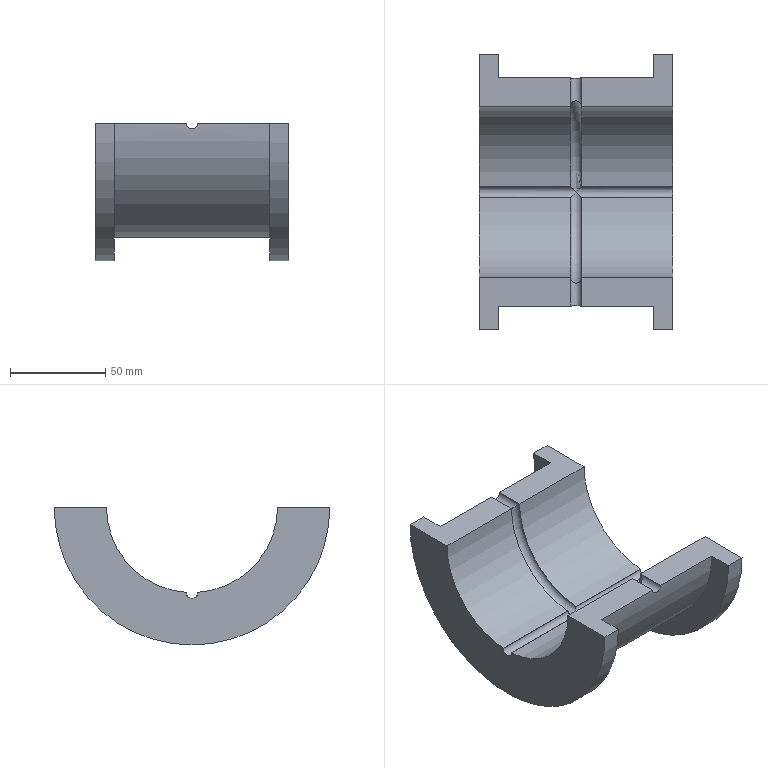Part | STEP file | Input 128 | 1 solid | 25 faces | box 102 x 145 x 72.5 mm | volume 300584 mm3 | cylinder 15 | plane 8 | torus 2 | commonest cylinder face diameters 6 x8 90 x4 145 x2 120 x1